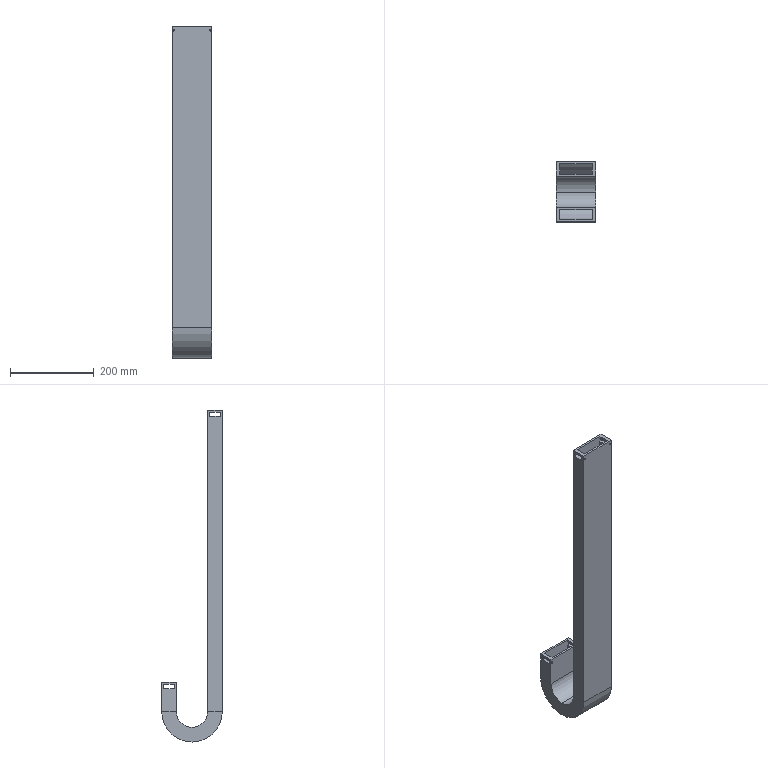Part | STEP file | 1 solid | 58 faces | box 94 x 145 x 792.5 mm | volume 1305245 mm3 | plane 34 | cylinder 24 | commonest cylinder face diameters 4 x16 75 x2 85 x2 135 x2 145 x2